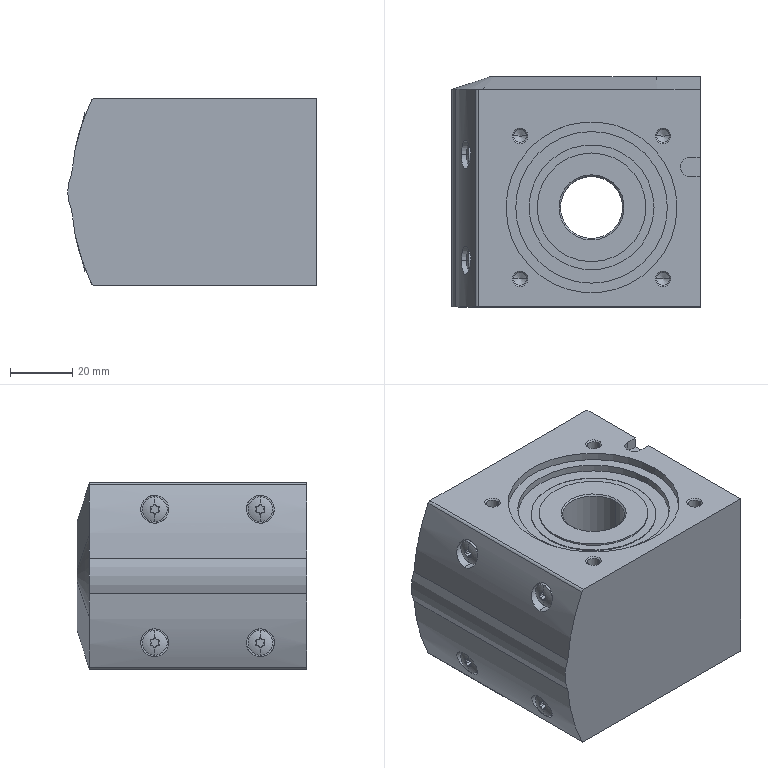Part | STEP file | _Endblock-SBG - PAS42 B 1 | 1 solid | 216 faces | box 80 x 74 x 60 mm | volume 295323 mm3 | cylinder 130 | cone 45 | plane 33 | torus 8 | commonest cylinder face diameters 0.644 x36 1.127 x32 4.134 x16 8 x8 9 x8 3.242 x4